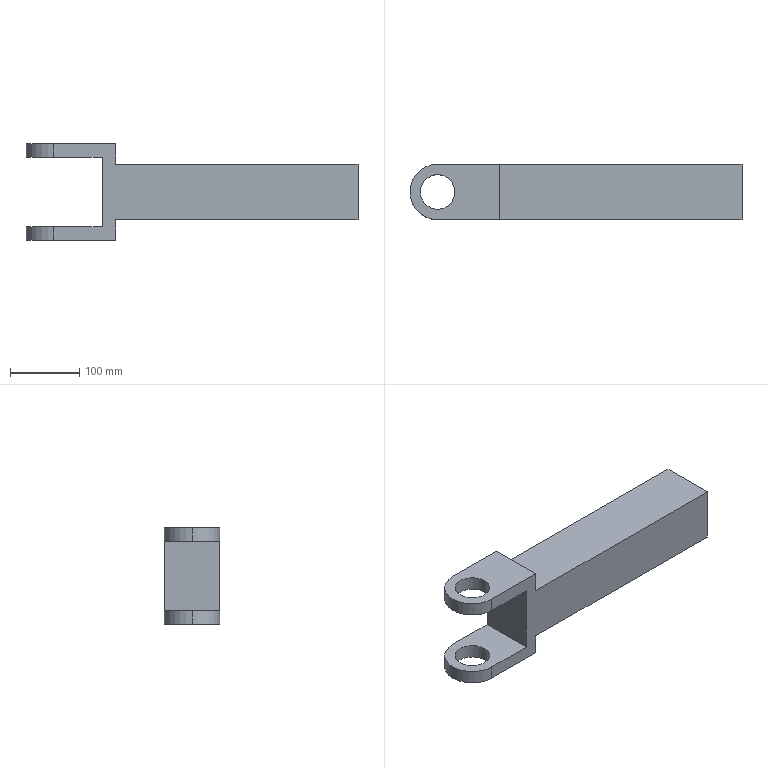Part | SolidWorks | 1 solid | 25 faces | box 480 x 80 x 140 mm | volume 1449991 mm3 | plane 17 | cylinder 8 | commonest cylinder face diameters 50 x4 80 x4
STEP:
#1=CARTESIAN_POINT('',(25.,0.,-50.));
#2=VERTEX_POINT('',#1);
#3=CARTESIAN_POINT('',(-25.,0.,-50.));
#4=VERTEX_POINT('',#3);
#5=CARTESIAN_POINT('',(0.,0.,-50.));
#6=DIRECTION('',(0.,0.,-1.));
#7=DIRECTION('',(-1.,0.,0.));
#8=AXIS2_PLACEMENT_3D('',#5,#6,#7);
#9=CIRCLE('',#8,25.);
#10=EDGE_CURVE('',#2,#4,#9,.T.);
#11=ORIENTED_EDGE('',*,*,#10,.F.);
#12=CARTESIAN_POINT('',(25.,0.,-70.));
#13=VERTEX_POINT('',#12);
#14=CARTESIAN_POINT('',(25.,0.,70.));
#15=DIRECTION('',(0.,0.,-1.));
#16=VECTOR('',#15,1000.);
#17=LINE('',#14,#16);
#18=EDGE_CURVE('',#2,#13,#17,.T.);
#19=ORIENTED_EDGE('',*,*,#18,.T.);
#20=CARTESIAN_POINT('',(-25.,0.,-70.));
#21=VERTEX_POINT('',#20);
#22=CARTESIAN_POINT('',(0.,0.,-70.));
#23=DIRECTION('',(0.,0.,1.));
#24=DIRECTION('',(1.,0.,0.));
#25=AXIS2_PLACEMENT_3D('',#22,#23,#24);
#26=CIRCLE('',#25,25.);
#27=EDGE_CURVE('',#21,#13,#26,.T.);
#28=ORIENTED_EDGE('',*,*,#27,.F.);
#29=CARTESIAN_POINT('',(-25.,0.,70.));
#30=DIRECTION('',(0.,0.,-1.));
#31=VECTOR('',#30,1000.);
#32=LINE('',#29,#31);
#33=EDGE_CURVE('',#4,#21,#32,.T.);
#34=ORIENTED_EDGE('',*,*,#33,.F.);
#35=EDGE_LOOP('',(#11,#19,#28,#34));
#36=FACE_OUTER_BOUND('',#35,.T.);
#37=CARTESIAN_POINT('',(0.,0.,70.));
#38=DIRECTION('',(0.,0.,-1.));
#39=DIRECTION('',(-1.,0.,0.));
#40=AXIS2_PLACEMENT_3D('',#37,#38,#39);
#41=CYLINDRICAL_SURFACE('',#40,25.);
#42=ADVANCED_FACE('',(#36),#41,.F.);
#43=CARTESIAN_POINT('',(0.,-40.,-50.));
#44=VERTEX_POINT('',#43);
#45=CARTESIAN_POINT('',(-40.,0.,-50.));
#46=VERTEX_POINT('',#45);
#47=CARTESIAN_POINT('',(0.,0.,-50.));
#48=DIRECTION('',(0.,0.,-1.));
#49=DIRECTION('',(-1.,0.,0.));
#50=AXIS2_PLACEMENT_3D('',#47,#48,#49);
#51=CIRCLE('',#50,40.);
#52=EDGE_CURVE('',#44,#46,#51,.T.);
#53=ORIENTED_EDGE('',*,*,#52,.T.);
#54=CARTESIAN_POINT('',(-40.,0.,-70.));
#55=VERTEX_POINT('',#54);
#56=CARTESIAN_POINT('',(-40.,0.,70.));
#57=DIRECTION('',(0.,0.,-1.));
#58=VECTOR('',#57,1000.);
#59=LINE('',#56,#58);
#60=EDGE_CURVE('',#46,#55,#59,.T.);
#61=ORIENTED_EDGE('',*,*,#60,.T.);
#62=CARTESIAN_POINT('',(0.,-40.,-70.));
#63=VERTEX_POINT('',#62);
#64=CARTESIAN_POINT('',(0.,0.,-70.));
#65=DIRECTION('',(0.,0.,1.));
#66=DIRECTION('',(1.,0.,0.));
#67=AXIS2_PLACEMENT_3D('',#64,#65,#66);
#68=CIRCLE('',#67,40.);
#69=EDGE_CURVE('',#55,#63,#68,.T.);
#70=ORIENTED_EDGE('',*,*,#69,.T.);
#71=CARTESIAN_POINT('',(0.,-40.,70.));
#72=DIRECTION('',(0.,0.,-1.));
#73=VECTOR('',#72,1000.);
#74=LINE('',#71,#73);
#75=EDGE_CURVE('',#44,#63,#74,.T.);
#76=ORIENTED_EDGE('',*,*,#75,.F.);
#77=EDGE_LOOP('',(#53,#61,#70,#76));
#78=FACE_OUTER_BOUND('',#77,.T.);
#79=CARTESIAN_POINT('',(0.,0.,70.));
#80=DIRECTION('',(0.,0.,-1.));
#81=DIRECTION('',(-1.,0.,0.));
#82=AXIS2_PLACEMENT_3D('',#79,#80,#81);
#83=CYLINDRICAL_SURFACE('',#82,40.);
#84=ADVANCED_FACE('',(#78),#83,.T.);
#85=CARTESIAN_POINT('',(-25.,0.,70.));
#86=VERTEX_POINT('',#85);
#87=CARTESIAN_POINT('',(25.,0.,70.));
#88=VERTEX_POINT('',#87);
#89=CARTESIAN_POINT('',(0.,0.,70.));
#90=DIRECTION('',(0.,0.,1.));
#91=DIRECTION('',(1.,0.,0.));
#92=AXIS2_PLACEMENT_3D('',#89,#90,#91);
#93=CIRCLE('',#92,25.);
#94=EDGE_CURVE('',#86,#88,#93,.T.);
#95=ORIENTED_EDGE('',*,*,#94,.T.);
#96=CARTESIAN_POINT('',(25.,0.,50.));
#97=VERTEX_POINT('',#96);
#98=CARTESIAN_POINT('',(25.,0.,70.));
#99=DIRECTION('',(0.,0.,-1.));
#100=VECTOR('',#99,1000.);
#101=LINE('',#98,#100);
#102=EDGE_CURVE('',#88,#97,#101,.T.);
#103=ORIENTED_EDGE('',*,*,#102,.T.);
#104=CARTESIAN_POINT('',(-25.,0.,50.));
#105=VERTEX_POINT('',#104);
#106=CARTESIAN_POINT('',(0.,0.,50.));
#107=DIRECTION('',(0.,0.,1.));
#108=DIRECTION('',(1.,0.,0.));
#109=AXIS2_PLACEMENT_3D('',#106,#107,#108);
#110=CIRCLE('',#109,25.);
#111=EDGE_CURVE('',#105,#97,#110,.T.);
#112=ORIENTED_EDGE('',*,*,#111,.F.);
#113=CARTESIAN_POINT('',(-25.,0.,70.));
#114=DIRECTION('',(0.,0.,-1.));
#115=VECTOR('',#114,1000.);
#116=LINE('',#113,#115);
#117=EDGE_CURVE('',#86,#105,#116,.T.);
#118=ORIENTED_EDGE('',*,*,#117,.F.);
#119=EDGE_LOOP('',(#95,#103,#112,#118));
#120=FACE_OUTER_BOUND('',#119,.T.);
#121=CARTESIAN_POINT('',(0.,0.,70.));
#122=DIRECTION('',(0.,0.,-1.));
#123=DIRECTION('',(-1.,0.,0.));
#124=AXIS2_PLACEMENT_3D('',#121,#122,#123);
#125=CYLINDRICAL_SURFACE('',#124,25.);
#126=ADVANCED_FACE('',(#120),#125,.F.);
#127=CARTESIAN_POINT('',(-40.,0.,70.));
#128=VERTEX_POINT('',#127);
#129=CARTESIAN_POINT('',(0.,-40.,70.));
#130=VERTEX_POINT('',#129);
#131=CARTESIAN_POINT('',(0.,0.,70.));
#132=DIRECTION('',(0.,0.,1.));
#133=DIRECTION('',(1.,0.,0.));
#134=AXIS2_PLACEMENT_3D('',#131,#132,#133);
#135=CIRCLE('',#134,40.);
#136=EDGE_CURVE('',#128,#130,#135,.T.);
#137=ORIENTED_EDGE('',*,*,#136,.F.);
#138=CARTESIAN_POINT('',(-40.,0.,50.));
#139=VERTEX_POINT('',#138);
#140=CARTESIAN_POINT('',(-40.,0.,70.));
#141=DIRECTION('',(0.,0.,-1.));
#142=VECTOR('',#141,1000.);
#143=LINE('',#140,#142);
#144=EDGE_CURVE('',#128,#139,#143,.T.);
#145=ORIENTED_EDGE('',*,*,#144,.T.);
#146=CARTESIAN_POINT('',(0.,-40.,50.));
#147=VERTEX_POINT('',#146);
#148=CARTESIAN_POINT('',(0.,0.,50.));
#149=DIRECTION('',(0.,0.,1.));
#150=DIRECTION('',(1.,0.,0.));
#151=AXIS2_PLACEMENT_3D('',#148,#149,#150);
#152=CIRCLE('',#151,40.);
#153=EDGE_CURVE('',#139,#147,#152,.T.);
#154=ORIENTED_EDGE('',*,*,#153,.T.);
#155=CARTESIAN_POINT('',(0.,-40.,70.));
#156=DIRECTION('',(0.,0.,-1.));
#157=VECTOR('',#156,1000.);
#158=LINE('',#155,#157);
#159=EDGE_CURVE('',#130,#147,#158,.T.);
#160=ORIENTED_EDGE('',*,*,#159,.F.);
#161=EDGE_LOOP('',(#137,#145,#154,#160));
#162=FACE_OUTER_BOUND('',#161,.T.);
#163=CARTESIAN_POINT('',(0.,0.,70.));
#164=DIRECTION('',(0.,0.,-1.));
#165=DIRECTION('',(-1.,0.,0.));
#166=AXIS2_PLACEMENT_3D('',#163,#164,#165);
#167=CYLINDRICAL_SURFACE('',#166,40.);
#168=ADVANCED_FACE('',(#162),#167,.T.);
#169=CARTESIAN_POINT('',(90.,-40.,-40.));
#170=VERTEX_POINT('',#169);
#171=CARTESIAN_POINT('',(90.,40.,-40.));
#172=VERTEX_POINT('',#171);
#173=CARTESIAN_POINT('',(90.,40.,-40.));
#174=DIRECTION('',(0.,1.,0.));
#175=VECTOR('',#174,1000.);
#176=LINE('',#173,#175);
#177=EDGE_CURVE('',#170,#172,#176,.T.);
#178=ORIENTED_EDGE('',*,*,#177,.F.);
#179=CARTESIAN_POINT('',(90.,-40.,-70.));
#180=VERTEX_POINT('',#179);
#181=CARTESIAN_POINT('',(90.,-40.,70.));
#182=DIRECTION('',(0.,0.,-1.));
#183=VECTOR('',#182,1000.);
#184=LINE('',#181,#183);
#185=EDGE_CURVE('',#170,#180,#184,.T.);
#186=ORIENTED_EDGE('',*,*,#185,.T.);
#187=CARTESIAN_POINT('',(90.,40.,-70.));
#188=VERTEX_POINT('',#187);
#189=CARTESIAN_POINT('',(90.,40.,-70.));
#190=DIRECTION('',(0.,1.,0.));
#191=VECTOR('',#190,1000.);
#192=LINE('',#189,#191);
#193=EDGE_CURVE('',#180,#188,#192,.T.);
#194=ORIENTED_EDGE('',*,*,#193,.T.);
#195=CARTESIAN_POINT('',(90.,40.,70.));
#196=DIRECTION('',(0.,0.,1.));
#197=VECTOR('',#196,1000.);
#198=LINE('',#195,#197);
#199=EDGE_CURVE('',#188,#172,#198,.T.);
#200=ORIENTED_EDGE('',*,*,#199,.T.);
#201=EDGE_LOOP('',(#178,#186,#194,#200));
#202=FACE_OUTER_BOUND('',#201,.T.);
#203=CARTESIAN_POINT('',(90.,0.,0.));
#204=DIRECTION('',(1.,0.,0.));
#205=DIRECTION('',(0.,0.,-1.));
#206=AXIS2_PLACEMENT_3D('',#203,#204,#205);
#207=PLANE('',#206);
#208=ADVANCED_FACE('',(#202),#207,.T.);
#209=CARTESIAN_POINT('',(70.,-40.,-50.));
#210=VERTEX_POINT('',#209);
#211=CARTESIAN_POINT('',(70.,40.,-50.));
#212=VERTEX_POINT('',#211);
#213=CARTESIAN_POINT('',(70.,-100.,-50.));
#214=DIRECTION('',(0.,1.,0.));
#215=VECTOR('',#214,1000.);
#216=LINE('',#213,#215);
#217=EDGE_CURVE('',#210,#212,#216,.T.);
#218=ORIENTED_EDGE('',*,*,#217,.F.);
#219=CARTESIAN_POINT('',(70.,-40.,50.));
#220=VERTEX_POINT('',#219);
#221=CARTESIAN_POINT('',(70.,-40.,70.));
#222=DIRECTION('',(0.,0.,-1.));
#223=VECTOR('',#222,1000.);
#224=LINE('',#221,#223);
#225=EDGE_CURVE('',#220,#210,#224,.T.);
#226=ORIENTED_EDGE('',*,*,#225,.F.);
#227=CARTESIAN_POINT('',(70.,40.,50.));
#228=VERTEX_POINT('',#227);
#229=CARTESIAN_POINT('',(70.,-100.,50.));
#230=DIRECTION('',(0.,1.,0.));
#231=VECTOR('',#230,1000.);
#232=LINE('',#229,#231);
#233=EDGE_CURVE('',#220,#228,#232,.T.);
#234=ORIENTED_EDGE('',*,*,#233,.T.);
#235=CARTESIAN_POINT('',(70.,40.,70.));
#236=DIRECTION('',(0.,0.,1.));
#237=VECTOR('',#236,1000.);
#238=LINE('',#235,#237);
#239=EDGE_CURVE('',#212,#228,#238,.T.);
#240=ORIENTED_EDGE('',*,*,#239,.F.);
#241=EDGE_LOOP('',(#218,#226,#234,#240));
#242=FACE_OUTER_BOUND('',#241,.T.);
#243=CARTESIAN_POINT('',(70.,0.,0.));
#244=DIRECTION('',(1.,0.,0.));
#245=DIRECTION('',(0.,0.,-1.));
#246=AXIS2_PLACEMENT_3D('',#243,#244,#245);
#247=PLANE('',#246);
#248=ADVANCED_FACE('',(#242),#247,.F.);
#249=ORIENTED_EDGE('',*,*,#159,.T.);
#250=CARTESIAN_POINT('',(0.,-40.,50.));
#251=DIRECTION('',(1.,0.,0.));
#252=VECTOR('',#251,1000.);
#253=LINE('',#250,#252);
#254=EDGE_CURVE('',#147,#220,#253,.T.);
#255=ORIENTED_EDGE('',*,*,#254,.T.);
#256=ORIENTED_EDGE('',*,*,#225,.T.);
#257=CARTESIAN_POINT('',(0.,-40.,-50.));
#258=DIRECTION('',(-1.,0.,0.));
#259=VECTOR('',#258,1000.);
#260=LINE('',#257,#259);
#261=EDGE_CURVE('',#210,#44,#260,.T.);
#262=ORIENTED_EDGE('',*,*,#261,.T.);
#263=ORIENTED_EDGE('',*,*,#75,.T.);
#264=CARTESIAN_POINT('',(90.,-40.,-70.));
#265=DIRECTION('',(-1.,0.,0.));
#266=VECTOR('',#265,1000.);
#267=LINE('',#264,#266);
#268=EDGE_CURVE('',#180,#63,#267,.T.);
#269=ORIENTED_EDGE('',*,*,#268,.F.);
#270=ORIENTED_EDGE('',*,*,#185,.F.);
#271=CARTESIAN_POINT('',(440.,-40.,-40.));
#272=VERTEX_POINT('',#271);
#273=CARTESIAN_POINT('',(440.,-40.,-40.));
#274=DIRECTION('',(-1.,0.,0.));
#275=VECTOR('',#274,1000.);
#276=LINE('',#273,#275);
#277=EDGE_CURVE('',#272,#170,#276,.T.);
#278=ORIENTED_EDGE('',*,*,#277,.F.);
#279=CARTESIAN_POINT('',(440.,-40.,40.));
#280=VERTEX_POINT('',#279);
#281=CARTESIAN_POINT('',(440.,-40.,40.));
#282=DIRECTION('',(0.,0.,-1.));
#283=VECTOR('',#282,1000.);
#284=LINE('',#281,#283);
#285=EDGE_CURVE('',#280,#272,#284,.T.);
#286=ORIENTED_EDGE('',*,*,#285,.F.);
#287=CARTESIAN_POINT('',(90.,-40.,40.));
#288=VERTEX_POINT('',#287);
#289=CARTESIAN_POINT('',(440.,-40.,40.));
#290=DIRECTION('',(-1.,0.,0.));
#291=VECTOR('',#290,1000.);
#292=LINE('',#289,#291);
#293=EDGE_CURVE('',#280,#288,#292,.T.);
#294=ORIENTED_EDGE('',*,*,#293,.T.);
#295=CARTESIAN_POINT('',(90.,-40.,70.));
#296=VERTEX_POINT('',#295);
#297=CARTESIAN_POINT('',(90.,-40.,70.));
#298=DIRECTION('',(0.,0.,-1.));
#299=VECTOR('',#298,1000.);
#300=LINE('',#297,#299);
#301=EDGE_CURVE('',#296,#288,#300,.T.);
#302=ORIENTED_EDGE('',*,*,#301,.F.);
#303=CARTESIAN_POINT('',(0.,-40.,70.));
#304=DIRECTION('',(1.,0.,0.));
#305=VECTOR('',#304,1000.);
#306=LINE('',#303,#305);
#307=EDGE_CURVE('',#130,#296,#306,.T.);
#308=ORIENTED_EDGE('',*,*,#307,.F.);
#309=EDGE_LOOP('',(#249,#255,#256,#262,#263,#269,#270,#278,#286,#294,#302,#308));
#310=FACE_OUTER_BOUND('',#309,.T.);
#311=CARTESIAN_POINT('',(0.,-40.,70.));
#312=DIRECTION('',(0.,1.,0.));
#313=DIRECTION('',(0.,0.,1.));
#314=AXIS2_PLACEMENT_3D('',#311,#312,#313);
#315=PLANE('',#314);
#316=ADVANCED_FACE('',(#310),#315,.F.);
#317=CARTESIAN_POINT('',(0.,40.,50.));
#318=VERTEX_POINT('',#317);
#319=CARTESIAN_POINT('',(-70.,40.,50.));
#320=DIRECTION('',(1.,0.,0.));
#321=VECTOR('',#320,1000.);
#322=LINE('',#319,#321);
#323=EDGE_CURVE('',#318,#228,#322,.T.);
#324=ORIENTED_EDGE('',*,*,#323,.F.);
#325=CARTESIAN_POINT('',(0.,40.,70.));
#326=VERTEX_POINT('',#325);
#327=CARTESIAN_POINT('',(0.,40.,70.));
#328=DIRECTION('',(0.,0.,-1.));
#329=VECTOR('',#328,1000.);
#330=LINE('',#327,#329);
#331=EDGE_CURVE('',#326,#318,#330,.T.);
#332=ORIENTED_EDGE('',*,*,#331,.F.);
#333=CARTESIAN_POINT('',(90.,40.,70.));
#334=VERTEX_POINT('',#333);
#335=CARTESIAN_POINT('',(0.,40.,70.));
#336=DIRECTION('',(1.,0.,0.));
#337=VECTOR('',#336,1000.);
#338=LINE('',#335,#337);
#339=EDGE_CURVE('',#326,#334,#338,.T.);
#340=ORIENTED_EDGE('',*,*,#339,.T.);
#341=CARTESIAN_POINT('',(90.,40.,40.));
#342=VERTEX_POINT('',#341);
#343=CARTESIAN_POINT('',(90.,40.,70.));
#344=DIRECTION('',(0.,0.,1.));
#345=VECTOR('',#344,1000.);
#346=LINE('',#343,#345);
#347=EDGE_CURVE('',#342,#334,#346,.T.);
#348=ORIENTED_EDGE('',*,*,#347,.F.);
#349=CARTESIAN_POINT('',(440.,40.,40.));
#350=VERTEX_POINT('',#349);
#351=CARTESIAN_POINT('',(440.,40.,40.));
#352=DIRECTION('',(-1.,0.,0.));
#353=VECTOR('',#352,1000.);
#354=LINE('',#351,#353);
#355=EDGE_CURVE('',#350,#342,#354,.T.);
#356=ORIENTED_EDGE('',*,*,#355,.F.);
#357=CARTESIAN_POINT('',(440.,40.,-40.));
#358=VERTEX_POINT('',#357);
#359=CARTESIAN_POINT('',(440.,40.,40.));
#360=DIRECTION('',(0.,0.,1.));
#361=VECTOR('',#360,1000.);
#362=LINE('',#359,#361);
#363=EDGE_CURVE('',#358,#350,#362,.T.);
#364=ORIENTED_EDGE('',*,*,#363,.F.);
#365=CARTESIAN_POINT('',(440.,40.,-40.));
#366=DIRECTION('',(-1.,0.,0.));
#367=VECTOR('',#366,1000.);
#368=LINE('',#365,#367);
#369=EDGE_CURVE('',#358,#172,#368,.T.);
#370=ORIENTED_EDGE('',*,*,#369,.T.);
#371=ORIENTED_EDGE('',*,*,#199,.F.);
#372=CARTESIAN_POINT('',(0.,40.,-70.));
#373=VERTEX_POINT('',#372);
#374=CARTESIAN_POINT('',(90.,40.,-70.));
#375=DIRECTION('',(-1.,0.,0.));
#376=VECTOR('',#375,1000.);
#377=LINE('',#374,#376);
#378=EDGE_CURVE('',#188,#373,#377,.T.);
#379=ORIENTED_EDGE('',*,*,#378,.T.);
#380=CARTESIAN_POINT('',(0.,40.,-50.));
#381=VERTEX_POINT('',#380);
#382=CARTESIAN_POINT('',(0.,40.,70.));
#383=DIRECTION('',(0.,0.,-1.));
#384=VECTOR('',#383,1000.);
#385=LINE('',#382,#384);
#386=EDGE_CURVE('',#381,#373,#385,.T.);
#387=ORIENTED_EDGE('',*,*,#386,.F.);
#388=CARTESIAN_POINT('',(-70.,40.,-50.));
#389=DIRECTION('',(-1.,0.,0.));
#390=VECTOR('',#389,1000.);
#391=LINE('',#388,#390);
#392=EDGE_CURVE('',#212,#381,#391,.T.);
#393=ORIENTED_EDGE('',*,*,#392,.F.);
#394=ORIENTED_EDGE('',*,*,#239,.T.);
#395=EDGE_LOOP('',(#324,#332,#340,#348,#356,#364,#370,#371,#379,#387,#393,#394));
#396=FACE_OUTER_BOUND('',#395,.T.);
#397=CARTESIAN_POINT('',(0.,40.,70.));
#398=DIRECTION('',(0.,1.,0.));
#399=DIRECTION('',(0.,0.,1.));
#400=AXIS2_PLACEMENT_3D('',#397,#398,#399);
#401=PLANE('',#400);
#402=ADVANCED_FACE('',(#396),#401,.T.);
#403=ORIENTED_EDGE('',*,*,#144,.F.);
#404=CARTESIAN_POINT('',(0.,0.,70.));
#405=DIRECTION('',(0.,0.,1.));
#406=DIRECTION('',(1.,0.,0.));
#407=AXIS2_PLACEMENT_3D('',#404,#405,#406);
#408=CIRCLE('',#407,40.);
#409=EDGE_CURVE('',#326,#128,#408,.T.);
#410=ORIENTED_EDGE('',*,*,#409,.F.);
#411=ORIENTED_EDGE('',*,*,#331,.T.);
#412=CARTESIAN_POINT('',(0.,0.,50.));
#413=DIRECTION('',(0.,0.,1.));
#414=DIRECTION('',(1.,0.,0.));
#415=AXIS2_PLACEMENT_3D('',#412,#413,#414);
#416=CIRCLE('',#415,40.);
#417=EDGE_CURVE('',#318,#139,#416,.T.);
#418=ORIENTED_EDGE('',*,*,#417,.T.);
#419=EDGE_LOOP('',(#403,#410,#411,#418));
#420=FACE_OUTER_BOUND('',#419,.T.);
#421=CARTESIAN_POINT('',(0.,0.,70.));
#422=DIRECTION('',(0.,0.,-1.));
#423=DIRECTION('',(-1.,0.,0.));
#424=AXIS2_PLACEMENT_3D('',#421,#422,#423);
#425=CYLINDRICAL_SURFACE('',#424,40.);
#426=ADVANCED_FACE('',(#420),#425,.T.);
#427=ORIENTED_EDGE('',*,*,#102,.F.);
#428=CARTESIAN_POINT('',(0.,0.,70.));
#429=DIRECTION('',(0.,0.,1.));
#430=DIRECTION('',(1.,0.,0.));
#431=AXIS2_PLACEMENT_3D('',#428,#429,#430);
#432=CIRCLE('',#431,25.);
#433=EDGE_CURVE('',#88,#86,#432,.T.);
#434=ORIENTED_EDGE('',*,*,#433,.T.);
#435=ORIENTED_EDGE('',*,*,#117,.T.);
#436=CARTESIAN_POINT('',(0.,0.,50.));
#437=DIRECTION('',(0.,0.,1.));
#438=DIRECTION('',(1.,0.,0.));
#439=AXIS2_PLACEMENT_3D('',#436,#437,#438);
#440=CIRCLE('',#439,25.);
#441=EDGE_CURVE('',#97,#105,#440,.T.);
#442=ORIENTED_EDGE('',*,*,#441,.F.);
#443=EDGE_LOOP('',(#427,#434,#435,#442));
#444=FACE_OUTER_BOUND('',#443,.T.);
#445=CARTESIAN_POINT('',(0.,0.,70.));
#446=DIRECTION('',(0.,0.,-1.));
#447=DIRECTION('',(-1.,0.,0.));
#448=AXIS2_PLACEMENT_3D('',#445,#446,#447);
#449=CYLINDRICAL_SURFACE('',#448,25.);
#450=ADVANCED_FACE('',(#444),#449,.F.);
#451=ORIENTED_EDGE('',*,*,#307,.T.);
#452=CARTESIAN_POINT('',(90.,40.,70.));
#453=DIRECTION('',(0.,-1.,0.));
#454=VECTOR('',#453,1000.);
#455=LINE('',#452,#454);
#456=EDGE_CURVE('',#334,#296,#455,.T.);
#457=ORIENTED_EDGE('',*,*,#456,.F.);
#458=ORIENTED_EDGE('',*,*,#339,.F.);
#459=ORIENTED_EDGE('',*,*,#409,.T.);
#460=ORIENTED_EDGE('',*,*,#136,.T.);
#461=EDGE_LOOP('',(#451,#457,#458,#459,#460));
#462=FACE_OUTER_BOUND('',#461,.T.);
#463=ORIENTED_EDGE('',*,*,#94,.F.);
#464=ORIENTED_EDGE('',*,*,#433,.F.);
#465=EDGE_LOOP('',(#463,#464));
#466=FACE_BOUND('',#465,.T.);
#467=CARTESIAN_POINT('',(0.,0.,70.));
#468=DIRECTION('',(0.,0.,1.));
#469=DIRECTION('',(1.,0.,0.));
#470=AXIS2_PLACEMENT_3D('',#467,#468,#469);
#471=PLANE('',#470);
#472=ADVANCED_FACE('',(#462,#466),#471,.T.);
#473=ORIENTED_EDGE('',*,*,#111,.T.);
#474=ORIENTED_EDGE('',*,*,#441,.T.);
#475=EDGE_LOOP('',(#473,#474));
#476=FACE_BOUND('',#475,.T.);
#477=ORIENTED_EDGE('',*,*,#417,.F.);
#478=ORIENTED_EDGE('',*,*,#323,.T.);
#479=ORIENTED_EDGE('',*,*,#233,.F.);
#480=ORIENTED_EDGE('',*,*,#254,.F.);
#481=ORIENTED_EDGE('',*,*,#153,.F.);
#482=EDGE_LOOP('',(#477,#478,#479,#480,#481));
#483=FACE_OUTER_BOUND('',#482,.T.);
#484=CARTESIAN_POINT('',(-70.,-100.,50.));
#485=DIRECTION('',(0.,0.,1.));
#486=DIRECTION('',(1.,0.,0.));
#487=AXIS2_PLACEMENT_3D('',#484,#485,#486);
#488=PLANE('',#487);
#489=ADVANCED_FACE('',(#476,#483),#488,.F.);
#490=ORIENTED_EDGE('',*,*,#268,.T.);
#491=ORIENTED_EDGE('',*,*,#69,.F.);
#492=CARTESIAN_POINT('',(0.,0.,-70.));
#493=DIRECTION('',(0.,0.,1.));
#494=DIRECTION('',(1.,0.,0.));
#495=AXIS2_PLACEMENT_3D('',#492,#493,#494);
#496=CIRCLE('',#495,40.);
#497=EDGE_CURVE('',#373,#55,#496,.T.);
#498=ORIENTED_EDGE('',*,*,#497,.F.);
#499=ORIENTED_EDGE('',*,*,#378,.F.);
#500=ORIENTED_EDGE('',*,*,#193,.F.);
#501=EDGE_LOOP('',(#490,#491,#498,#499,#500));
#502=FACE_OUTER_BOUND('',#501,.T.);
#503=ORIENTED_EDGE('',*,*,#27,.T.);
#504=CARTESIAN_POINT('',(0.,0.,-70.));
#505=DIRECTION('',(0.,0.,1.));
#506=DIRECTION('',(1.,0.,0.));
#507=AXIS2_PLACEMENT_3D('',#504,#505,#506);
#508=CIRCLE('',#507,25.);
#509=EDGE_CURVE('',#13,#21,#508,.T.);
#510=ORIENTED_EDGE('',*,*,#509,.T.);
#511=EDGE_LOOP('',(#503,#510));
#512=FACE_BOUND('',#511,.T.);
#513=CARTESIAN_POINT('',(90.,40.,-70.));
#514=DIRECTION('',(0.,0.,1.));
#515=DIRECTION('',(1.,0.,0.));
#516=AXIS2_PLACEMENT_3D('',#513,#514,#515);
#517=PLANE('',#516);
#518=ADVANCED_FACE('',(#502,#512),#517,.F.);
#519=CARTESIAN_POINT('',(90.,40.,40.));
#520=DIRECTION('',(0.,-1.,0.));
#521=VECTOR('',#520,1000.);
#522=LINE('',#519,#521);
#523=EDGE_CURVE('',#342,#288,#522,.T.);
#524=ORIENTED_EDGE('',*,*,#523,.F.);
#525=ORIENTED_EDGE('',*,*,#347,.T.);
#526=ORIENTED_EDGE('',*,*,#456,.T.);
#527=ORIENTED_EDGE('',*,*,#301,.T.);
#528=EDGE_LOOP('',(#524,#525,#526,#527));
#529=FACE_OUTER_BOUND('',#528,.T.);
#530=CARTESIAN_POINT('',(90.,0.,0.));
#531=DIRECTION('',(1.,0.,0.));
#532=DIRECTION('',(0.,0.,-1.));
#533=AXIS2_PLACEMENT_3D('',#530,#531,#532);
#534=PLANE('',#533);
#535=ADVANCED_FACE('',(#529),#534,.T.);
#536=ORIENTED_EDGE('',*,*,#60,.F.);
#537=CARTESIAN_POINT('',(0.,0.,-50.));
#538=DIRECTION('',(0.,0.,-1.));
#539=DIRECTION('',(-1.,0.,0.));
#540=AXIS2_PLACEMENT_3D('',#537,#538,#539);
#541=CIRCLE('',#540,40.);
#542=EDGE_CURVE('',#46,#381,#541,.T.);
#543=ORIENTED_EDGE('',*,*,#542,.T.);
#544=ORIENTED_EDGE('',*,*,#386,.T.);
#545=ORIENTED_EDGE('',*,*,#497,.T.);
#546=EDGE_LOOP('',(#536,#543,#544,#545));
#547=FACE_OUTER_BOUND('',#546,.T.);
#548=CARTESIAN_POINT('',(0.,0.,70.));
#549=DIRECTION('',(0.,0.,-1.));
#550=DIRECTION('',(-1.,0.,0.));
#551=AXIS2_PLACEMENT_3D('',#548,#549,#550);
#552=CYLINDRICAL_SURFACE('',#551,40.);
#553=ADVANCED_FACE('',(#547),#552,.T.);
#554=ORIENTED_EDGE('',*,*,#18,.F.);
#555=CARTESIAN_POINT('',(0.,0.,-50.));
#556=DIRECTION('',(0.,0.,-1.));
#557=DIRECTION('',(-1.,0.,0.));
#558=AXIS2_PLACEMENT_3D('',#555,#556,#557);
#559=CIRCLE('',#558,25.);
#560=EDGE_CURVE('',#4,#2,#559,.T.);
#561=ORIENTED_EDGE('',*,*,#560,.F.);
#562=ORIENTED_EDGE('',*,*,#33,.T.);
#563=ORIENTED_EDGE('',*,*,#509,.F.);
#564=EDGE_LOOP('',(#554,#561,#562,#563));
#565=FACE_OUTER_BOUND('',#564,.T.);
#566=CARTESIAN_POINT('',(0.,0.,70.));
#567=DIRECTION('',(0.,0.,-1.));
#568=DIRECTION('',(-1.,0.,0.));
#569=AXIS2_PLACEMENT_3D('',#566,#567,#568);
#570=CYLINDRICAL_SURFACE('',#569,25.);
#571=ADVANCED_FACE('',(#565),#570,.F.);
#572=ORIENTED_EDGE('',*,*,#560,.T.);
#573=ORIENTED_EDGE('',*,*,#10,.T.);
#574=EDGE_LOOP('',(#572,#573));
#575=FACE_BOUND('',#574,.T.);
#576=ORIENTED_EDGE('',*,*,#217,.T.);
#577=ORIENTED_EDGE('',*,*,#392,.T.);
#578=ORIENTED_EDGE('',*,*,#542,.F.);
#579=ORIENTED_EDGE('',*,*,#52,.F.);
#580=ORIENTED_EDGE('',*,*,#261,.F.);
#581=EDGE_LOOP('',(#576,#577,#578,#579,#580));
#582=FACE_OUTER_BOUND('',#581,.T.);
#583=CARTESIAN_POINT('',(-70.,-100.,-50.));
#584=DIRECTION('',(0.,0.,-1.));
#585=DIRECTION('',(-1.,0.,0.));
#586=AXIS2_PLACEMENT_3D('',#583,#584,#585);
#587=PLANE('',#586);
#588=ADVANCED_FACE('',(#575,#582),#587,.F.);
#589=ORIENTED_EDGE('',*,*,#177,.T.);
#590=ORIENTED_EDGE('',*,*,#369,.F.);
#591=CARTESIAN_POINT('',(440.,40.,-40.));
#592=DIRECTION('',(0.,1.,0.));
#593=VECTOR('',#592,1000.);
#594=LINE('',#591,#593);
#595=EDGE_CURVE('',#272,#358,#594,.T.);
#596=ORIENTED_EDGE('',*,*,#595,.F.);
#597=ORIENTED_EDGE('',*,*,#277,.T.);
#598=EDGE_LOOP('',(#589,#590,#596,#597));
#599=FACE_OUTER_BOUND('',#598,.T.);
#600=CARTESIAN_POINT('',(440.,40.,-40.));
#601=DIRECTION('',(0.,0.,1.));
#602=DIRECTION('',(1.,0.,0.));
#603=AXIS2_PLACEMENT_3D('',#600,#601,#602);
#604=PLANE('',#603);
#605=ADVANCED_FACE('',(#599),#604,.F.);
#606=ORIENTED_EDGE('',*,*,#523,.T.);
#607=ORIENTED_EDGE('',*,*,#293,.F.);
#608=CARTESIAN_POINT('',(440.,40.,40.));
#609=DIRECTION('',(0.,-1.,0.));
#610=VECTOR('',#609,1000.);
#611=LINE('',#608,#610);
#612=EDGE_CURVE('',#350,#280,#611,.T.);
#613=ORIENTED_EDGE('',*,*,#612,.F.);
#614=ORIENTED_EDGE('',*,*,#355,.T.);
#615=EDGE_LOOP('',(#606,#607,#613,#614));
#616=FACE_OUTER_BOUND('',#615,.T.);
#617=CARTESIAN_POINT('',(440.,40.,40.));
#618=DIRECTION('',(0.,0.,-1.));
#619=DIRECTION('',(-1.,0.,0.));
#620=AXIS2_PLACEMENT_3D('',#617,#618,#619);
#621=PLANE('',#620);
#622=ADVANCED_FACE('',(#616),#621,.F.);
#623=CARTESIAN_POINT('',(440.,-30.,30.));
#624=VERTEX_POINT('',#623);
#625=CARTESIAN_POINT('',(440.,-30.,-30.));
#626=VERTEX_POINT('',#625);
#627=CARTESIAN_POINT('',(440.,-30.,30.));
#628=DIRECTION('',(0.,0.,-1.));
#629=VECTOR('',#628,1000.);
#630=LINE('',#627,#629);
#631=EDGE_CURVE('',#624,#626,#630,.T.);
#632=ORIENTED_EDGE('',*,*,#631,.F.);
#633=CARTESIAN_POINT('',(440.,30.,30.));
#634=VERTEX_POINT('',#633);
#635=CARTESIAN_POINT('',(440.,30.,30.));
#636=DIRECTION('',(0.,-1.,0.));
#637=VECTOR('',#636,1000.);
#638=LINE('',#635,#637);
#639=EDGE_CURVE('',#634,#624,#638,.T.);
#640=ORIENTED_EDGE('',*,*,#639,.F.);
#641=CARTESIAN_POINT('',(440.,30.,-30.));
#642=VERTEX_POINT('',#641);
#643=CARTESIAN_POINT('',(440.,30.,-30.));
#644=DIRECTION('',(0.,0.,1.));
#645=VECTOR('',#644,1000.);
#646=LINE('',#643,#645);
#647=EDGE_CURVE('',#642,#634,#646,.T.);
#648=ORIENTED_EDGE('',*,*,#647,.F.);
#649=CARTESIAN_POINT('',(440.,-30.,-30.));
#650=DIRECTION('',(0.,1.,0.));
#651=VECTOR('',#650,1000.);
#652=LINE('',#649,#651);
#653=EDGE_CURVE('',#626,#642,#652,.T.);
#654=ORIENTED_EDGE('',*,*,#653,.F.);
#655=EDGE_LOOP('',(#632,#640,#648,#654));
#656=FACE_BOUND('',#655,.T.);
#657=ORIENTED_EDGE('',*,*,#595,.T.);
#658=ORIENTED_EDGE('',*,*,#363,.T.);
#659=ORIENTED_EDGE('',*,*,#612,.T.);
#660=ORIENTED_EDGE('',*,*,#285,.T.);
#661=EDGE_LOOP('',(#657,#658,#659,#660));
#662=FACE_OUTER_BOUND('',#661,.T.);
#663=CARTESIAN_POINT('',(440.,0.,0.));
#664=DIRECTION('',(1.,0.,0.));
#665=DIRECTION('',(0.,0.,-1.));
#666=AXIS2_PLACEMENT_3D('',#663,#664,#665);
#667=PLANE('',#666);
#668=ADVANCED_FACE('',(#656,#662),#667,.T.);
#669=CARTESIAN_POINT('',(90.,-30.,-30.));
#670=VERTEX_POINT('',#669);
#671=CARTESIAN_POINT('',(90.,-30.,30.));
#672=VERTEX_POINT('',#671);
#673=CARTESIAN_POINT('',(90.,-30.,30.));
#674=DIRECTION('',(0.,0.,1.));
#675=VECTOR('',#674,1000.);
#676=LINE('',#673,#675);
#677=EDGE_CURVE('',#670,#672,#676,.T.);
#678=ORIENTED_EDGE('',*,*,#677,.T.);
#679=CARTESIAN_POINT('',(5.147,-30.,30.));
#680=DIRECTION('',(1.,0.,0.));
#681=VECTOR('',#680,1000.);
#682=LINE('',#679,#681);
#683=EDGE_CURVE('',#672,#624,#682,.T.);
#684=ORIENTED_EDGE('',*,*,#683,.T.);
#685=ORIENTED_EDGE('',*,*,#631,.T.);
#686=CARTESIAN_POINT('',(5.147,-30.,-30.));
#687=DIRECTION('',(1.,0.,0.));
#688=VECTOR('',#687,1000.);
#689=LINE('',#686,#688);
#690=EDGE_CURVE('',#670,#626,#689,.T.);
#691=ORIENTED_EDGE('',*,*,#690,.F.);
#692=EDGE_LOOP('',(#678,#684,#685,#691));
#693=FACE_OUTER_BOUND('',#692,.T.);
#694=CARTESIAN_POINT('',(5.147,-30.,30.));
#695=DIRECTION('',(0.,-1.,0.));
#696=DIRECTION('',(0.,0.,-1.));
#697=AXIS2_PLACEMENT_3D('',#694,#695,#696);
#698=PLANE('',#697);
#699=ADVANCED_FACE('',(#693),#698,.F.);
#700=CARTESIAN_POINT('',(90.,30.,30.));
#701=VERTEX_POINT('',#700);
#702=CARTESIAN_POINT('',(90.,30.,30.));
#703=DIRECTION('',(0.,1.,0.));
#704=VECTOR('',#703,1000.);
#705=LINE('',#702,#704);
#706=EDGE_CURVE('',#672,#701,#705,.T.);
#707=ORIENTED_EDGE('',*,*,#706,.T.);
#708=CARTESIAN_POINT('',(5.147,30.,30.));
#709=DIRECTION('',(1.,0.,0.));
#710=VECTOR('',#709,1000.);
#711=LINE('',#708,#710);
#712=EDGE_CURVE('',#701,#634,#711,.T.);
#713=ORIENTED_EDGE('',*,*,#712,.T.);
#714=ORIENTED_EDGE('',*,*,#639,.T.);
#715=ORIENTED_EDGE('',*,*,#683,.F.);
#716=EDGE_LOOP('',(#707,#713,#714,#715));
#717=FACE_OUTER_BOUND('',#716,.T.);
#718=CARTESIAN_POINT('',(5.147,30.,30.));
#719=DIRECTION('',(0.,0.,1.));
#720=DIRECTION('',(1.,0.,0.));
#721=AXIS2_PLACEMENT_3D('',#718,#719,#720);
#722=PLANE('',#721);
#723=ADVANCED_FACE('',(#717),#722,.F.);
#724=CARTESIAN_POINT('',(90.,30.,-30.));
#725=VERTEX_POINT('',#724);
#726=CARTESIAN_POINT('',(90.,30.,-30.));
#727=DIRECTION('',(0.,0.,-1.));
#728=VECTOR('',#727,1000.);
#729=LINE('',#726,#728);
#730=EDGE_CURVE('',#701,#725,#729,.T.);
#731=ORIENTED_EDGE('',*,*,#730,.T.);
#732=CARTESIAN_POINT('',(5.147,30.,-30.));
#733=DIRECTION('',(1.,0.,0.));
#734=VECTOR('',#733,1000.);
#735=LINE('',#732,#734);
#736=EDGE_CURVE('',#725,#642,#735,.T.);
#737=ORIENTED_EDGE('',*,*,#736,.T.);
#738=ORIENTED_EDGE('',*,*,#647,.T.);
#739=ORIENTED_EDGE('',*,*,#712,.F.);
#740=EDGE_LOOP('',(#731,#737,#738,#739));
#741=FACE_OUTER_BOUND('',#740,.T.);
#742=CARTESIAN_POINT('',(5.147,30.,-30.));
#743=DIRECTION('',(0.,1.,0.));
#744=DIRECTION('',(0.,0.,1.));
#745=AXIS2_PLACEMENT_3D('',#742,#743,#744);
#746=PLANE('',#745);
#747=ADVANCED_FACE('',(#741),#746,.F.);
#748=CARTESIAN_POINT('',(90.,-30.,-30.));
#749=DIRECTION('',(0.,-1.,0.));
#750=VECTOR('',#749,1000.);
#751=LINE('',#748,#750);
#752=EDGE_CURVE('',#725,#670,#751,.T.);
#753=ORIENTED_EDGE('',*,*,#752,.T.);
#754=ORIENTED_EDGE('',*,*,#690,.T.);
#755=ORIENTED_EDGE('',*,*,#653,.T.);
#756=ORIENTED_EDGE('',*,*,#736,.F.);
#757=EDGE_LOOP('',(#753,#754,#755,#756));
#758=FACE_OUTER_BOUND('',#757,.T.);
#759=CARTESIAN_POINT('',(5.147,-30.,-30.));
#760=DIRECTION('',(0.,0.,-1.));
#761=DIRECTION('',(-1.,0.,0.));
#762=AXIS2_PLACEMENT_3D('',#759,#760,#761);
#763=PLANE('',#762);
#764=ADVANCED_FACE('',(#758),#763,.F.);
#765=ORIENTED_EDGE('',*,*,#677,.F.);
#766=ORIENTED_EDGE('',*,*,#752,.F.);
#767=ORIENTED_EDGE('',*,*,#730,.F.);
#768=ORIENTED_EDGE('',*,*,#706,.F.);
#769=EDGE_LOOP('',(#765,#766,#767,#768));
#770=FACE_OUTER_BOUND('',#769,.T.);
#771=CARTESIAN_POINT('',(90.,0.,0.));
#772=DIRECTION('',(1.,0.,0.));
#773=DIRECTION('',(0.,0.,-1.));
#774=AXIS2_PLACEMENT_3D('',#771,#772,#773);
#775=PLANE('',#774);
#776=ADVANCED_FACE('',(#770),#775,.T.);
#777=CLOSED_SHELL('',(#42,#84,#126,#168,#208,#248,#316,#402,#426,#450,#472,#489,#518,#535,#553,#571,#588,#605,#622,#668,#699,#723,#747,#764,#776));
#778=MANIFOLD_SOLID_BREP('',#777);
#779=CARTESIAN_POINT('',(0.,0.,0.));
#780=DIRECTION('',(0.,0.,1.));
#781=DIRECTION('',(1.,0.,0.));
#782=AXIS2_PLACEMENT_3D('',#779,#780,#781);
#783=(LENGTH_UNIT()NAMED_UNIT(*)SI_UNIT(.MILLI.,.METRE.));
#784=UNCERTAINTY_MEASURE_WITH_UNIT(LENGTH_MEASURE(0.00001),#783,'','');
#785=(NAMED_UNIT(*)PLANE_ANGLE_UNIT()SI_UNIT($,.RADIAN.));
#786=(NAMED_UNIT(*)SI_UNIT($,.STERADIAN.)SOLID_ANGLE_UNIT());
#787=(GEOMETRIC_REPRESENTATION_CONTEXT(3)GLOBAL_UNCERTAINTY_ASSIGNED_CONTEXT((#784))GLOBAL_UNIT_ASSIGNED_CONTEXT((#783,#785,#786))REPRESENTATION_CONTEXT('',''));
#788=ADVANCED_BREP_SHAPE_REPRESENTATION('',(#778,#782),#787);